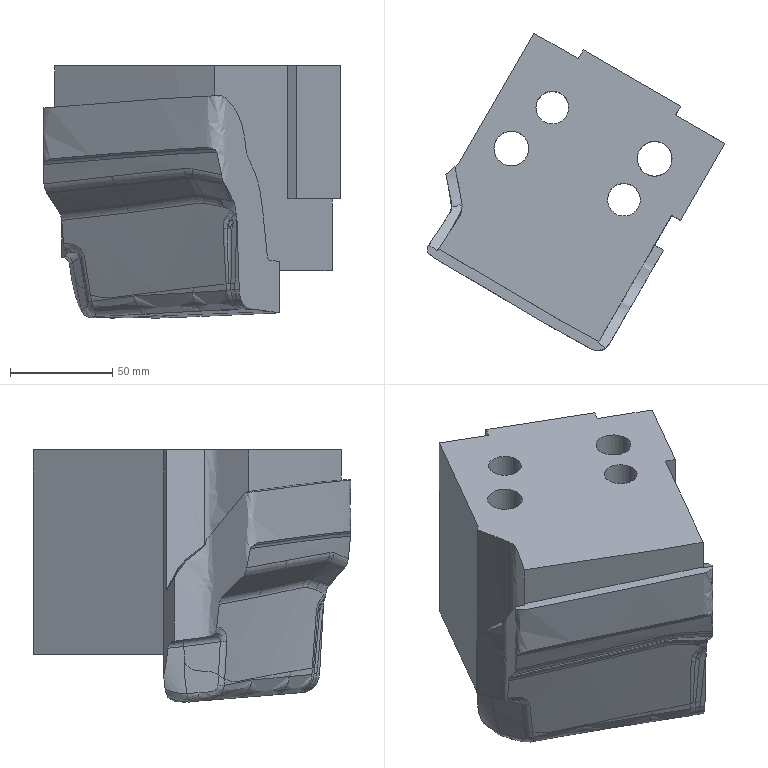Part | NX | features solid 2 | 1 solid | 89 faces | box 145.53 x 155.186 x 123.982 mm | volume 1117833 mm3 | spline 64 | plane 17 | cylinder 8 | commonest cylinder face diameters 16 x2 17 x2 25 x2 8 x1 10 x1